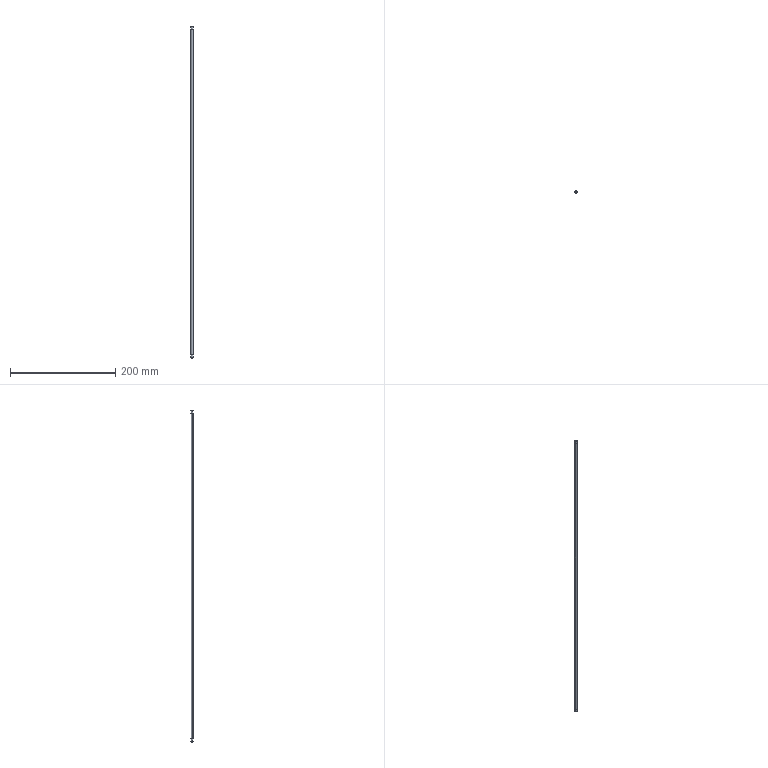Part | SolidWorks | features Chamfer 1, Extrusion 1, ICE 1, MirrorPattern 1 | 1 solid | 16 faces | box 5 x 5 x 632 mm | volume 12318 mm3 | cone 8 | cylinder 6 | plane 2 | commonest cylinder face diameters 4 x4 5 x2
STEP:
#1=CARTESIAN_POINT('',(1.5,0.,316.));
#2=VERTEX_POINT('',#1);
#3=CARTESIAN_POINT('',(-1.5,0.,316.));
#4=VERTEX_POINT('',#3);
#5=CARTESIAN_POINT('',(0.,0.,316.));
#6=DIRECTION('',(0.,0.,1.));
#7=DIRECTION('',(1.,0.,0.));
#8=AXIS2_PLACEMENT_3D('',#5,#6,#7);
#9=CIRCLE('',#8,1.5);
#10=EDGE_CURVE('',#2,#4,#9,.T.);
#11=ORIENTED_EDGE('',*,*,#10,.F.);
#12=CARTESIAN_POINT('',(2.,0.,315.5));
#13=VERTEX_POINT('',#12);
#14=CARTESIAN_POINT('',(1.5,0.,316.));
#15=DIRECTION('',(0.7071,0.,-0.7071));
#16=VECTOR('',#15,1000.);
#17=LINE('',#14,#16);
#18=EDGE_CURVE('',#2,#13,#17,.T.);
#19=ORIENTED_EDGE('',*,*,#18,.T.);
#20=CARTESIAN_POINT('',(-2.,0.,315.5));
#21=VERTEX_POINT('',#20);
#22=CARTESIAN_POINT('',(0.,0.,315.5));
#23=DIRECTION('',(0.,0.,-1.));
#24=DIRECTION('',(1.,0.,0.));
#25=AXIS2_PLACEMENT_3D('',#22,#23,#24);
#26=CIRCLE('',#25,2.);
#27=EDGE_CURVE('',#21,#13,#26,.T.);
#28=ORIENTED_EDGE('',*,*,#27,.F.);
#29=CARTESIAN_POINT('',(-1.5,0.,316.));
#30=DIRECTION('',(-0.7071,0.,-0.7071));
#31=VECTOR('',#30,1000.);
#32=LINE('',#29,#31);
#33=EDGE_CURVE('',#4,#21,#32,.T.);
#34=ORIENTED_EDGE('',*,*,#33,.F.);
#35=EDGE_LOOP('',(#11,#19,#28,#34));
#36=FACE_OUTER_BOUND('',#35,.T.);
#37=CARTESIAN_POINT('',(0.,0.,316.));
#38=DIRECTION('',(0.,0.,-1.));
#39=DIRECTION('',(-1.,0.,0.));
#40=AXIS2_PLACEMENT_3D('',#37,#38,#39);
#41=CONICAL_SURFACE('',#40,1.5,0.7854);
#42=ADVANCED_FACE('',(#36),#41,.T.);
#43=CARTESIAN_POINT('',(2.,0.,310.));
#44=VERTEX_POINT('',#43);
#45=CARTESIAN_POINT('',(-2.,0.,310.));
#46=VERTEX_POINT('',#45);
#47=CARTESIAN_POINT('',(0.,0.,310.));
#48=DIRECTION('',(0.,0.,1.));
#49=DIRECTION('',(1.,0.,0.));
#50=AXIS2_PLACEMENT_3D('',#47,#48,#49);
#51=CIRCLE('',#50,2.);
#52=EDGE_CURVE('',#44,#46,#51,.T.);
#53=ORIENTED_EDGE('',*,*,#52,.F.);
#54=CARTESIAN_POINT('',(2.5,0.,309.5));
#55=VERTEX_POINT('',#54);
#56=CARTESIAN_POINT('',(2.,0.,310.));
#57=DIRECTION('',(0.7071,0.,-0.7071));
#58=VECTOR('',#57,1000.);
#59=LINE('',#56,#58);
#60=EDGE_CURVE('',#44,#55,#59,.T.);
#61=ORIENTED_EDGE('',*,*,#60,.T.);
#62=CARTESIAN_POINT('',(-2.5,0.,309.5));
#63=VERTEX_POINT('',#62);
#64=CARTESIAN_POINT('',(0.,0.,309.5));
#65=DIRECTION('',(0.,0.,-1.));
#66=DIRECTION('',(1.,0.,0.));
#67=AXIS2_PLACEMENT_3D('',#64,#65,#66);
#68=CIRCLE('',#67,2.5);
#69=EDGE_CURVE('',#63,#55,#68,.T.);
#70=ORIENTED_EDGE('',*,*,#69,.F.);
#71=CARTESIAN_POINT('',(-2.,0.,310.));
#72=DIRECTION('',(-0.7071,0.,-0.7071));
#73=VECTOR('',#72,1000.);
#74=LINE('',#71,#73);
#75=EDGE_CURVE('',#46,#63,#74,.T.);
#76=ORIENTED_EDGE('',*,*,#75,.F.);
#77=EDGE_LOOP('',(#53,#61,#70,#76));
#78=FACE_OUTER_BOUND('',#77,.T.);
#79=CARTESIAN_POINT('',(0.,0.,310.));
#80=DIRECTION('',(0.,0.,-1.));
#81=DIRECTION('',(-1.,0.,0.));
#82=AXIS2_PLACEMENT_3D('',#79,#80,#81);
#83=CONICAL_SURFACE('',#82,2.,0.7854);
#84=ADVANCED_FACE('',(#78),#83,.T.);
#85=CARTESIAN_POINT('',(2.,0.,-310.));
#86=VERTEX_POINT('',#85);
#87=CARTESIAN_POINT('',(-2.,0.,-310.));
#88=VERTEX_POINT('',#87);
#89=CARTESIAN_POINT('',(0.,0.,-310.));
#90=DIRECTION('',(0.,0.,1.));
#91=DIRECTION('',(1.,0.,0.));
#92=AXIS2_PLACEMENT_3D('',#89,#90,#91);
#93=CIRCLE('',#92,2.);
#94=EDGE_CURVE('',#86,#88,#93,.T.);
#95=ORIENTED_EDGE('',*,*,#94,.T.);
#96=CARTESIAN_POINT('',(-2.5,0.,-309.5));
#97=VERTEX_POINT('',#96);
#98=CARTESIAN_POINT('',(-2.5,0.,-309.5));
#99=DIRECTION('',(-0.7071,0.,0.7071));
#100=VECTOR('',#99,1000.);
#101=LINE('',#98,#100);
#102=EDGE_CURVE('',#88,#97,#101,.T.);
#103=ORIENTED_EDGE('',*,*,#102,.T.);
#104=CARTESIAN_POINT('',(2.5,0.,-309.5));
#105=VERTEX_POINT('',#104);
#106=CARTESIAN_POINT('',(0.,0.,-309.5));
#107=DIRECTION('',(0.,0.,1.));
#108=DIRECTION('',(1.,0.,0.));
#109=AXIS2_PLACEMENT_3D('',#106,#107,#108);
#110=CIRCLE('',#109,2.5);
#111=EDGE_CURVE('',#105,#97,#110,.T.);
#112=ORIENTED_EDGE('',*,*,#111,.F.);
#113=CARTESIAN_POINT('',(2.5,0.,-309.5));
#114=DIRECTION('',(0.7071,0.,0.7071));
#115=VECTOR('',#114,1000.);
#116=LINE('',#113,#115);
#117=EDGE_CURVE('',#86,#105,#116,.T.);
#118=ORIENTED_EDGE('',*,*,#117,.F.);
#119=EDGE_LOOP('',(#95,#103,#112,#118));
#120=FACE_OUTER_BOUND('',#119,.T.);
#121=CARTESIAN_POINT('',(0.,0.,-309.5));
#122=DIRECTION('',(0.,0.,1.));
#123=DIRECTION('',(1.,0.,0.));
#124=AXIS2_PLACEMENT_3D('',#121,#122,#123);
#125=CONICAL_SURFACE('',#124,2.5,0.7854);
#126=ADVANCED_FACE('',(#120),#125,.T.);
#127=CARTESIAN_POINT('',(-1.5,0.,-316.));
#128=VERTEX_POINT('',#127);
#129=CARTESIAN_POINT('',(1.5,0.,-316.));
#130=VERTEX_POINT('',#129);
#131=CARTESIAN_POINT('',(0.,0.,-316.));
#132=DIRECTION('',(0.,0.,-1.));
#133=DIRECTION('',(-1.,0.,0.));
#134=AXIS2_PLACEMENT_3D('',#131,#132,#133);
#135=CIRCLE('',#134,1.5);
#136=EDGE_CURVE('',#128,#130,#135,.T.);
#137=ORIENTED_EDGE('',*,*,#136,.F.);
#138=CARTESIAN_POINT('',(-2.,0.,-315.5));
#139=VERTEX_POINT('',#138);
#140=CARTESIAN_POINT('',(-2.,0.,-315.5));
#141=DIRECTION('',(-0.7071,0.,0.7071));
#142=VECTOR('',#141,1000.);
#143=LINE('',#140,#142);
#144=EDGE_CURVE('',#128,#139,#143,.T.);
#145=ORIENTED_EDGE('',*,*,#144,.T.);
#146=CARTESIAN_POINT('',(2.,0.,-315.5));
#147=VERTEX_POINT('',#146);
#148=CARTESIAN_POINT('',(0.,0.,-315.5));
#149=DIRECTION('',(0.,0.,1.));
#150=DIRECTION('',(-1.,0.,0.));
#151=AXIS2_PLACEMENT_3D('',#148,#149,#150);
#152=CIRCLE('',#151,2.);
#153=EDGE_CURVE('',#147,#139,#152,.T.);
#154=ORIENTED_EDGE('',*,*,#153,.F.);
#155=CARTESIAN_POINT('',(2.,0.,-315.5));
#156=DIRECTION('',(0.7071,0.,0.7071));
#157=VECTOR('',#156,1000.);
#158=LINE('',#155,#157);
#159=EDGE_CURVE('',#130,#147,#158,.T.);
#160=ORIENTED_EDGE('',*,*,#159,.F.);
#161=EDGE_LOOP('',(#137,#145,#154,#160));
#162=FACE_OUTER_BOUND('',#161,.T.);
#163=CARTESIAN_POINT('',(0.,0.,-315.5));
#164=DIRECTION('',(0.,0.,1.));
#165=DIRECTION('',(1.,0.,0.));
#166=AXIS2_PLACEMENT_3D('',#163,#164,#165);
#167=CONICAL_SURFACE('',#166,2.,0.7854);
#168=ADVANCED_FACE('',(#162),#167,.T.);
#169=ORIENTED_EDGE('',*,*,#153,.T.);
#170=CARTESIAN_POINT('',(-2.,0.,-316.));
#171=DIRECTION('',(0.,0.,1.));
#172=VECTOR('',#171,1000.);
#173=LINE('',#170,#172);
#174=EDGE_CURVE('',#139,#88,#173,.T.);
#175=ORIENTED_EDGE('',*,*,#174,.T.);
#176=ORIENTED_EDGE('',*,*,#94,.F.);
#177=CARTESIAN_POINT('',(2.,0.,-316.));
#178=DIRECTION('',(0.,0.,1.));
#179=VECTOR('',#178,1000.);
#180=LINE('',#177,#179);
#181=EDGE_CURVE('',#147,#86,#180,.T.);
#182=ORIENTED_EDGE('',*,*,#181,.F.);
#183=EDGE_LOOP('',(#169,#175,#176,#182));
#184=FACE_OUTER_BOUND('',#183,.T.);
#185=CARTESIAN_POINT('',(0.,0.,-316.));
#186=DIRECTION('',(0.,0.,1.));
#187=DIRECTION('',(1.,0.,0.));
#188=AXIS2_PLACEMENT_3D('',#185,#186,#187);
#189=CYLINDRICAL_SURFACE('',#188,2.);
#190=ADVANCED_FACE('',(#184),#189,.T.);
#191=ORIENTED_EDGE('',*,*,#27,.T.);
#192=CARTESIAN_POINT('',(2.,0.,316.));
#193=DIRECTION('',(0.,0.,-1.));
#194=VECTOR('',#193,1000.);
#195=LINE('',#192,#194);
#196=EDGE_CURVE('',#13,#44,#195,.T.);
#197=ORIENTED_EDGE('',*,*,#196,.T.);
#198=ORIENTED_EDGE('',*,*,#52,.T.);
#199=CARTESIAN_POINT('',(-2.,0.,316.));
#200=DIRECTION('',(0.,0.,-1.));
#201=VECTOR('',#200,1000.);
#202=LINE('',#199,#201);
#203=EDGE_CURVE('',#21,#46,#202,.T.);
#204=ORIENTED_EDGE('',*,*,#203,.F.);
#205=EDGE_LOOP('',(#191,#197,#198,#204));
#206=FACE_OUTER_BOUND('',#205,.T.);
#207=CARTESIAN_POINT('',(0.,0.,316.));
#208=DIRECTION('',(0.,0.,-1.));
#209=DIRECTION('',(-1.,0.,0.));
#210=AXIS2_PLACEMENT_3D('',#207,#208,#209);
#211=CYLINDRICAL_SURFACE('',#210,2.);
#212=ADVANCED_FACE('',(#206),#211,.T.);
#213=ORIENTED_EDGE('',*,*,#69,.T.);
#214=CARTESIAN_POINT('',(2.5,0.,310.));
#215=DIRECTION('',(0.,0.,-1.));
#216=VECTOR('',#215,1000.);
#217=LINE('',#214,#216);
#218=EDGE_CURVE('',#55,#105,#217,.T.);
#219=ORIENTED_EDGE('',*,*,#218,.T.);
#220=ORIENTED_EDGE('',*,*,#111,.T.);
#221=CARTESIAN_POINT('',(-2.5,0.,310.));
#222=DIRECTION('',(0.,0.,-1.));
#223=VECTOR('',#222,1000.);
#224=LINE('',#221,#223);
#225=EDGE_CURVE('',#63,#97,#224,.T.);
#226=ORIENTED_EDGE('',*,*,#225,.F.);
#227=EDGE_LOOP('',(#213,#219,#220,#226));
#228=FACE_OUTER_BOUND('',#227,.T.);
#229=CARTESIAN_POINT('',(0.,0.,310.));
#230=DIRECTION('',(0.,0.,-1.));
#231=DIRECTION('',(-1.,0.,0.));
#232=AXIS2_PLACEMENT_3D('',#229,#230,#231);
#233=CYLINDRICAL_SURFACE('',#232,2.5);
#234=ADVANCED_FACE('',(#228),#233,.T.);
#235=ORIENTED_EDGE('',*,*,#218,.F.);
#236=CARTESIAN_POINT('',(0.,0.,309.5));
#237=DIRECTION('',(0.,0.,-1.));
#238=DIRECTION('',(1.,0.,0.));
#239=AXIS2_PLACEMENT_3D('',#236,#237,#238);
#240=CIRCLE('',#239,2.5);
#241=EDGE_CURVE('',#55,#63,#240,.T.);
#242=ORIENTED_EDGE('',*,*,#241,.T.);
#243=ORIENTED_EDGE('',*,*,#225,.T.);
#244=CARTESIAN_POINT('',(0.,0.,-309.5));
#245=DIRECTION('',(0.,0.,1.));
#246=DIRECTION('',(1.,0.,0.));
#247=AXIS2_PLACEMENT_3D('',#244,#245,#246);
#248=CIRCLE('',#247,2.5);
#249=EDGE_CURVE('',#97,#105,#248,.T.);
#250=ORIENTED_EDGE('',*,*,#249,.T.);
#251=EDGE_LOOP('',(#235,#242,#243,#250));
#252=FACE_OUTER_BOUND('',#251,.T.);
#253=CARTESIAN_POINT('',(0.,0.,310.));
#254=DIRECTION('',(0.,0.,-1.));
#255=DIRECTION('',(-1.,0.,0.));
#256=AXIS2_PLACEMENT_3D('',#253,#254,#255);
#257=CYLINDRICAL_SURFACE('',#256,2.5);
#258=ADVANCED_FACE('',(#252),#257,.T.);
#259=ORIENTED_EDGE('',*,*,#196,.F.);
#260=CARTESIAN_POINT('',(0.,0.,315.5));
#261=DIRECTION('',(0.,0.,-1.));
#262=DIRECTION('',(1.,0.,0.));
#263=AXIS2_PLACEMENT_3D('',#260,#261,#262);
#264=CIRCLE('',#263,2.);
#265=EDGE_CURVE('',#13,#21,#264,.T.);
#266=ORIENTED_EDGE('',*,*,#265,.T.);
#267=ORIENTED_EDGE('',*,*,#203,.T.);
#268=CARTESIAN_POINT('',(0.,0.,310.));
#269=DIRECTION('',(0.,0.,1.));
#270=DIRECTION('',(1.,0.,0.));
#271=AXIS2_PLACEMENT_3D('',#268,#269,#270);
#272=CIRCLE('',#271,2.);
#273=EDGE_CURVE('',#46,#44,#272,.T.);
#274=ORIENTED_EDGE('',*,*,#273,.T.);
#275=EDGE_LOOP('',(#259,#266,#267,#274));
#276=FACE_OUTER_BOUND('',#275,.T.);
#277=CARTESIAN_POINT('',(0.,0.,316.));
#278=DIRECTION('',(0.,0.,-1.));
#279=DIRECTION('',(-1.,0.,0.));
#280=AXIS2_PLACEMENT_3D('',#277,#278,#279);
#281=CYLINDRICAL_SURFACE('',#280,2.);
#282=ADVANCED_FACE('',(#276),#281,.T.);
#283=CARTESIAN_POINT('',(0.,0.,316.));
#284=DIRECTION('',(0.,0.,1.));
#285=DIRECTION('',(1.,0.,0.));
#286=AXIS2_PLACEMENT_3D('',#283,#284,#285);
#287=CIRCLE('',#286,1.5);
#288=EDGE_CURVE('',#4,#2,#287,.T.);
#289=ORIENTED_EDGE('',*,*,#288,.T.);
#290=ORIENTED_EDGE('',*,*,#10,.T.);
#291=EDGE_LOOP('',(#289,#290));
#292=FACE_OUTER_BOUND('',#291,.T.);
#293=CARTESIAN_POINT('',(0.,0.,316.));
#294=DIRECTION('',(0.,0.,1.));
#295=DIRECTION('',(1.,0.,0.));
#296=AXIS2_PLACEMENT_3D('',#293,#294,#295);
#297=PLANE('',#296);
#298=ADVANCED_FACE('',(#292),#297,.T.);
#299=ORIENTED_EDGE('',*,*,#174,.F.);
#300=CARTESIAN_POINT('',(0.,0.,-315.5));
#301=DIRECTION('',(0.,0.,1.));
#302=DIRECTION('',(-1.,0.,0.));
#303=AXIS2_PLACEMENT_3D('',#300,#301,#302);
#304=CIRCLE('',#303,2.);
#305=EDGE_CURVE('',#139,#147,#304,.T.);
#306=ORIENTED_EDGE('',*,*,#305,.T.);
#307=ORIENTED_EDGE('',*,*,#181,.T.);
#308=CARTESIAN_POINT('',(0.,0.,-310.));
#309=DIRECTION('',(0.,0.,1.));
#310=DIRECTION('',(1.,0.,0.));
#311=AXIS2_PLACEMENT_3D('',#308,#309,#310);
#312=CIRCLE('',#311,2.);
#313=EDGE_CURVE('',#88,#86,#312,.T.);
#314=ORIENTED_EDGE('',*,*,#313,.F.);
#315=EDGE_LOOP('',(#299,#306,#307,#314));
#316=FACE_OUTER_BOUND('',#315,.T.);
#317=CARTESIAN_POINT('',(0.,0.,-316.));
#318=DIRECTION('',(0.,0.,1.));
#319=DIRECTION('',(1.,0.,0.));
#320=AXIS2_PLACEMENT_3D('',#317,#318,#319);
#321=CYLINDRICAL_SURFACE('',#320,2.);
#322=ADVANCED_FACE('',(#316),#321,.T.);
#323=CARTESIAN_POINT('',(0.,0.,-316.));
#324=DIRECTION('',(0.,0.,-1.));
#325=DIRECTION('',(-1.,0.,0.));
#326=AXIS2_PLACEMENT_3D('',#323,#324,#325);
#327=CIRCLE('',#326,1.5);
#328=EDGE_CURVE('',#130,#128,#327,.T.);
#329=ORIENTED_EDGE('',*,*,#328,.T.);
#330=ORIENTED_EDGE('',*,*,#136,.T.);
#331=EDGE_LOOP('',(#329,#330));
#332=FACE_OUTER_BOUND('',#331,.T.);
#333=CARTESIAN_POINT('',(0.,0.,-316.));
#334=DIRECTION('',(0.,0.,-1.));
#335=DIRECTION('',(1.,0.,0.));
#336=AXIS2_PLACEMENT_3D('',#333,#334,#335);
#337=PLANE('',#336);
#338=ADVANCED_FACE('',(#332),#337,.T.);
#339=ORIENTED_EDGE('',*,*,#144,.F.);
#340=ORIENTED_EDGE('',*,*,#328,.F.);
#341=ORIENTED_EDGE('',*,*,#159,.T.);
#342=ORIENTED_EDGE('',*,*,#305,.F.);
#343=EDGE_LOOP('',(#339,#340,#341,#342));
#344=FACE_OUTER_BOUND('',#343,.T.);
#345=CARTESIAN_POINT('',(0.,0.,-315.5));
#346=DIRECTION('',(0.,0.,1.));
#347=DIRECTION('',(1.,0.,0.));
#348=AXIS2_PLACEMENT_3D('',#345,#346,#347);
#349=CONICAL_SURFACE('',#348,2.,0.7854);
#350=ADVANCED_FACE('',(#344),#349,.T.);
#351=ORIENTED_EDGE('',*,*,#102,.F.);
#352=ORIENTED_EDGE('',*,*,#313,.T.);
#353=ORIENTED_EDGE('',*,*,#117,.T.);
#354=ORIENTED_EDGE('',*,*,#249,.F.);
#355=EDGE_LOOP('',(#351,#352,#353,#354));
#356=FACE_OUTER_BOUND('',#355,.T.);
#357=CARTESIAN_POINT('',(0.,0.,-309.5));
#358=DIRECTION('',(0.,0.,1.));
#359=DIRECTION('',(1.,0.,0.));
#360=AXIS2_PLACEMENT_3D('',#357,#358,#359);
#361=CONICAL_SURFACE('',#360,2.5,0.7854);
#362=ADVANCED_FACE('',(#356),#361,.T.);
#363=ORIENTED_EDGE('',*,*,#60,.F.);
#364=ORIENTED_EDGE('',*,*,#273,.F.);
#365=ORIENTED_EDGE('',*,*,#75,.T.);
#366=ORIENTED_EDGE('',*,*,#241,.F.);
#367=EDGE_LOOP('',(#363,#364,#365,#366));
#368=FACE_OUTER_BOUND('',#367,.T.);
#369=CARTESIAN_POINT('',(0.,0.,310.));
#370=DIRECTION('',(0.,0.,-1.));
#371=DIRECTION('',(-1.,0.,0.));
#372=AXIS2_PLACEMENT_3D('',#369,#370,#371);
#373=CONICAL_SURFACE('',#372,2.,0.7854);
#374=ADVANCED_FACE('',(#368),#373,.T.);
#375=ORIENTED_EDGE('',*,*,#18,.F.);
#376=ORIENTED_EDGE('',*,*,#288,.F.);
#377=ORIENTED_EDGE('',*,*,#33,.T.);
#378=ORIENTED_EDGE('',*,*,#265,.F.);
#379=EDGE_LOOP('',(#375,#376,#377,#378));
#380=FACE_OUTER_BOUND('',#379,.T.);
#381=CARTESIAN_POINT('',(0.,0.,316.));
#382=DIRECTION('',(0.,0.,-1.));
#383=DIRECTION('',(-1.,0.,0.));
#384=AXIS2_PLACEMENT_3D('',#381,#382,#383);
#385=CONICAL_SURFACE('',#384,1.5,0.7854);
#386=ADVANCED_FACE('',(#380),#385,.T.);
#387=CLOSED_SHELL('',(#42,#84,#126,#168,#190,#212,#234,#258,#282,#298,#322,#338,#350,#362,#374,#386));
#388=MANIFOLD_SOLID_BREP('',#387);
#389=CARTESIAN_POINT('',(0.,0.,0.));
#390=DIRECTION('',(0.,0.,1.));
#391=DIRECTION('',(1.,0.,0.));
#392=AXIS2_PLACEMENT_3D('',#389,#390,#391);
#393=(LENGTH_UNIT()NAMED_UNIT(*)SI_UNIT(.MILLI.,.METRE.));
#394=UNCERTAINTY_MEASURE_WITH_UNIT(LENGTH_MEASURE(0.00001),#393,'','');
#395=(NAMED_UNIT(*)PLANE_ANGLE_UNIT()SI_UNIT($,.RADIAN.));
#396=(NAMED_UNIT(*)SI_UNIT($,.STERADIAN.)SOLID_ANGLE_UNIT());
#397=(GEOMETRIC_REPRESENTATION_CONTEXT(3)GLOBAL_UNCERTAINTY_ASSIGNED_CONTEXT((#394))GLOBAL_UNIT_ASSIGNED_CONTEXT((#393,#395,#396))REPRESENTATION_CONTEXT('',''));
#398=ADVANCED_BREP_SHAPE_REPRESENTATION('',(#388,#392),#397);